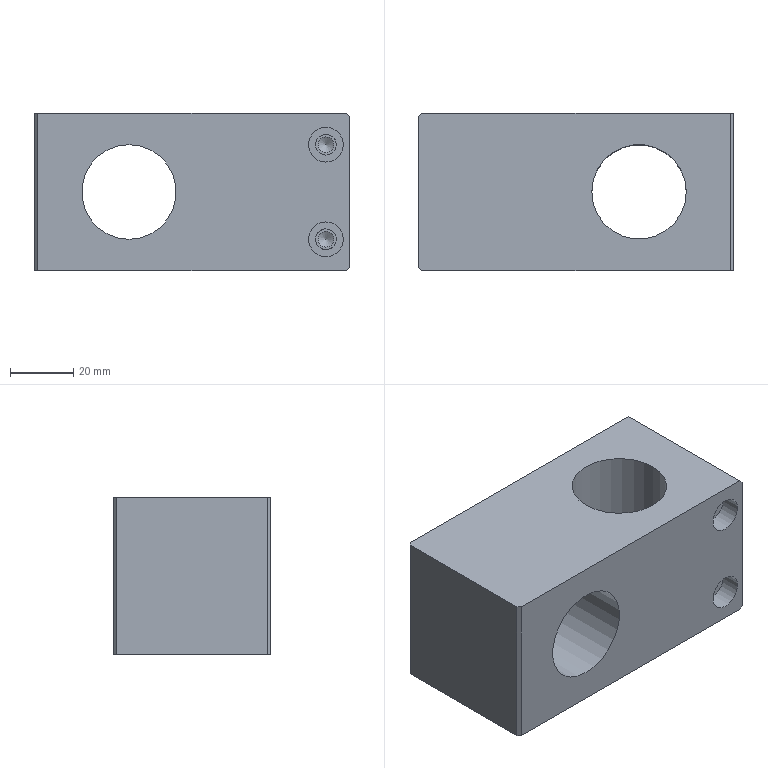Part | NX | 1 solid | 36 faces | box 100 x 50 x 50 mm | volume 172813 mm3 | plane 18 | cylinder 14 | cone 4 | commonest cylinder face diameters 5 x4 6.6 x4 11 x4 30 x2
STEP:
#1=CARTESIAN_POINT('',(42.5,1.5,7.5));
#2=VERTEX_POINT('',#1);
#3=CARTESIAN_POINT('',(42.5,1.5,10.));
#4=DIRECTION('',(0.,-1.,0.));
#5=DIRECTION('',(0.,0.,-1.));
#6=AXIS2_PLACEMENT_3D('',#3,#4,#5);
#7=CIRCLE('',#6,2.5);
#8=EDGE_CURVE('',#2,#2,#7,.T.);
#9=ORIENTED_EDGE('',*,*,#8,.F.);
#10=EDGE_LOOP('',(#9));
#11=FACE_BOUND('',#10,.T.);
#12=CARTESIAN_POINT('',(39.2,1.5,10.));
#13=VERTEX_POINT('',#12);
#14=CARTESIAN_POINT('',(42.5,1.5,10.));
#15=DIRECTION('',(0.,1.,0.));
#16=DIRECTION('',(-1.,0.,0.));
#17=AXIS2_PLACEMENT_3D('',#14,#15,#16);
#18=CIRCLE('',#17,3.3);
#19=EDGE_CURVE('',#13,#13,#18,.T.);
#20=ORIENTED_EDGE('',*,*,#19,.F.);
#21=EDGE_LOOP('',(#20));
#22=FACE_BOUND('',#21,.T.);
#23=CARTESIAN_POINT('',(0.,1.5,50.));
#24=DIRECTION('',(0.,1.,0.));
#25=DIRECTION('',(-1.,0.,0.));
#26=AXIS2_PLACEMENT_3D('',#23,#24,#25);
#27=PLANE('',#26);
#28=ADVANCED_FACE('',(#11,#22),#27,.F.);
#29=CARTESIAN_POINT('',(42.5,1.5,37.5));
#30=VERTEX_POINT('',#29);
#31=CARTESIAN_POINT('',(42.5,1.5,40.));
#32=DIRECTION('',(0.,-1.,0.));
#33=DIRECTION('',(0.,0.,-1.));
#34=AXIS2_PLACEMENT_3D('',#31,#32,#33);
#35=CIRCLE('',#34,2.5);
#36=EDGE_CURVE('',#30,#30,#35,.T.);
#37=ORIENTED_EDGE('',*,*,#36,.F.);
#38=EDGE_LOOP('',(#37));
#39=FACE_BOUND('',#38,.T.);
#40=CARTESIAN_POINT('',(39.2,1.5,40.));
#41=VERTEX_POINT('',#40);
#42=CARTESIAN_POINT('',(42.5,1.5,40.));
#43=DIRECTION('',(0.,1.,0.));
#44=DIRECTION('',(-1.,0.,0.));
#45=AXIS2_PLACEMENT_3D('',#42,#43,#44);
#46=CIRCLE('',#45,3.3);
#47=EDGE_CURVE('',#41,#41,#46,.T.);
#48=ORIENTED_EDGE('',*,*,#47,.F.);
#49=EDGE_LOOP('',(#48));
#50=FACE_BOUND('',#49,.T.);
#51=CARTESIAN_POINT('',(0.,1.5,50.));
#52=DIRECTION('',(0.,1.,0.));
#53=DIRECTION('',(-1.,0.,0.));
#54=AXIS2_PLACEMENT_3D('',#51,#52,#53);
#55=PLANE('',#54);
#56=ADVANCED_FACE('',(#39,#50),#55,.F.);
#57=CARTESIAN_POINT('',(-45.,15.,26.5));
#58=VERTEX_POINT('',#57);
#59=CARTESIAN_POINT('',(-42.5,15.,26.5));
#60=DIRECTION('',(0.,0.,-1.));
#61=DIRECTION('',(-1.,0.,0.));
#62=AXIS2_PLACEMENT_3D('',#59,#60,#61);
#63=CIRCLE('',#62,2.5);
#64=EDGE_CURVE('',#58,#58,#63,.T.);
#65=ORIENTED_EDGE('',*,*,#64,.F.);
#66=EDGE_LOOP('',(#65));
#67=FACE_BOUND('',#66,.T.);
#68=CARTESIAN_POINT('',(-39.2,15.,26.5));
#69=VERTEX_POINT('',#68);
#70=CARTESIAN_POINT('',(-42.5,15.,26.5));
#71=DIRECTION('',(0.,0.,1.));
#72=DIRECTION('',(1.,0.,0.));
#73=AXIS2_PLACEMENT_3D('',#70,#71,#72);
#74=CIRCLE('',#73,3.3);
#75=EDGE_CURVE('',#69,#69,#74,.F.);
#76=ORIENTED_EDGE('',*,*,#75,.T.);
#77=EDGE_LOOP('',(#76));
#78=FACE_BOUND('',#77,.T.);
#79=CARTESIAN_POINT('',(-50.,25.,26.5));
#80=DIRECTION('',(0.,0.,1.));
#81=DIRECTION('',(1.,0.,0.));
#82=AXIS2_PLACEMENT_3D('',#79,#80,#81);
#83=PLANE('',#82);
#84=ADVANCED_FACE('',(#67,#78),#83,.F.);
#85=CARTESIAN_POINT('',(-45.,-15.,26.5));
#86=VERTEX_POINT('',#85);
#87=CARTESIAN_POINT('',(-42.5,-15.,26.5));
#88=DIRECTION('',(0.,0.,-1.));
#89=DIRECTION('',(-1.,0.,0.));
#90=AXIS2_PLACEMENT_3D('',#87,#88,#89);
#91=CIRCLE('',#90,2.5);
#92=EDGE_CURVE('',#86,#86,#91,.T.);
#93=ORIENTED_EDGE('',*,*,#92,.F.);
#94=EDGE_LOOP('',(#93));
#95=FACE_BOUND('',#94,.T.);
#96=CARTESIAN_POINT('',(-39.2,-15.,26.5));
#97=VERTEX_POINT('',#96);
#98=CARTESIAN_POINT('',(-42.5,-15.,26.5));
#99=DIRECTION('',(0.,0.,1.));
#100=DIRECTION('',(1.,0.,0.));
#101=AXIS2_PLACEMENT_3D('',#98,#99,#100);
#102=CIRCLE('',#101,3.3);
#103=EDGE_CURVE('',#97,#97,#102,.F.);
#104=ORIENTED_EDGE('',*,*,#103,.T.);
#105=EDGE_LOOP('',(#104));
#106=FACE_BOUND('',#105,.T.);
#107=CARTESIAN_POINT('',(-50.,25.,26.5));
#108=DIRECTION('',(0.,0.,1.));
#109=DIRECTION('',(1.,0.,0.));
#110=AXIS2_PLACEMENT_3D('',#107,#108,#109);
#111=PLANE('',#110);
#112=ADVANCED_FACE('',(#95,#106),#111,.F.);
#113=CARTESIAN_POINT('',(-50.,24.,0.));
#114=VERTEX_POINT('',#113);
#115=CARTESIAN_POINT('',(-49.,25.,0.));
#116=VERTEX_POINT('',#115);
#117=CARTESIAN_POINT('',(-37.,37.,0.));
#118=DIRECTION('',(0.7071,0.7071,0.));
#119=VECTOR('',#118,1000.);
#120=LINE('',#117,#119);
#121=EDGE_CURVE('',#114,#116,#120,.T.);
#122=ORIENTED_EDGE('',*,*,#121,.F.);
#123=CARTESIAN_POINT('',(-50.,24.,50.));
#124=VERTEX_POINT('',#123);
#125=CARTESIAN_POINT('',(-50.,24.,50.));
#126=DIRECTION('',(0.,0.,-1.));
#127=VECTOR('',#126,1000.);
#128=LINE('',#125,#127);
#129=EDGE_CURVE('',#124,#114,#128,.T.);
#130=ORIENTED_EDGE('',*,*,#129,.F.);
#131=CARTESIAN_POINT('',(-49.,25.,50.));
#132=VERTEX_POINT('',#131);
#133=CARTESIAN_POINT('',(-50.,24.,50.));
#134=DIRECTION('',(-0.7071,-0.7071,0.));
#135=VECTOR('',#134,1000.);
#136=LINE('',#133,#135);
#137=EDGE_CURVE('',#132,#124,#136,.T.);
#138=ORIENTED_EDGE('',*,*,#137,.F.);
#139=CARTESIAN_POINT('',(-49.,25.,50.));
#140=DIRECTION('',(0.,0.,1.));
#141=VECTOR('',#140,1000.);
#142=LINE('',#139,#141);
#143=EDGE_CURVE('',#116,#132,#142,.T.);
#144=ORIENTED_EDGE('',*,*,#143,.F.);
#145=EDGE_LOOP('',(#122,#130,#138,#144));
#146=FACE_BOUND('',#145,.T.);
#147=CARTESIAN_POINT('',(-50.,24.,50.));
#148=DIRECTION('',(0.7071,-0.7071,0.));
#149=DIRECTION('',(0.,0.,-1.));
#150=AXIS2_PLACEMENT_3D('',#147,#148,#149);
#151=PLANE('',#150);
#152=ADVANCED_FACE('',(#146),#151,.F.);
#153=CARTESIAN_POINT('',(-49.,-25.,0.));
#154=VERTEX_POINT('',#153);
#155=CARTESIAN_POINT('',(-50.,-24.,0.));
#156=VERTEX_POINT('',#155);
#157=CARTESIAN_POINT('',(-37.,-37.,0.));
#158=DIRECTION('',(-0.7071,0.7071,0.));
#159=VECTOR('',#158,1000.);
#160=LINE('',#157,#159);
#161=EDGE_CURVE('',#154,#156,#160,.T.);
#162=ORIENTED_EDGE('',*,*,#161,.F.);
#163=CARTESIAN_POINT('',(-49.,-25.,50.));
#164=VERTEX_POINT('',#163);
#165=CARTESIAN_POINT('',(-49.,-25.,50.));
#166=DIRECTION('',(0.,0.,-1.));
#167=VECTOR('',#166,1000.);
#168=LINE('',#165,#167);
#169=EDGE_CURVE('',#164,#154,#168,.T.);
#170=ORIENTED_EDGE('',*,*,#169,.F.);
#171=CARTESIAN_POINT('',(-50.,-24.,50.));
#172=VERTEX_POINT('',#171);
#173=CARTESIAN_POINT('',(-49.,-25.,50.));
#174=DIRECTION('',(0.7071,-0.7071,0.));
#175=VECTOR('',#174,1000.);
#176=LINE('',#173,#175);
#177=EDGE_CURVE('',#172,#164,#176,.T.);
#178=ORIENTED_EDGE('',*,*,#177,.F.);
#179=CARTESIAN_POINT('',(-50.,-24.,50.));
#180=DIRECTION('',(0.,0.,1.));
#181=VECTOR('',#180,1000.);
#182=LINE('',#179,#181);
#183=EDGE_CURVE('',#156,#172,#182,.T.);
#184=ORIENTED_EDGE('',*,*,#183,.F.);
#185=EDGE_LOOP('',(#162,#170,#178,#184));
#186=FACE_BOUND('',#185,.T.);
#187=CARTESIAN_POINT('',(-49.,-25.,50.));
#188=DIRECTION('',(0.7071,0.7071,0.));
#189=DIRECTION('',(0.,0.,-1.));
#190=AXIS2_PLACEMENT_3D('',#187,#188,#189);
#191=PLANE('',#190);
#192=ADVANCED_FACE('',(#186),#191,.F.);
#193=CARTESIAN_POINT('',(49.,-25.,50.));
#194=VERTEX_POINT('',#193);
#195=CARTESIAN_POINT('',(49.,25.,50.));
#196=VERTEX_POINT('',#195);
#197=CARTESIAN_POINT('',(49.,0.,50.));
#198=DIRECTION('',(0.,1.,0.));
#199=VECTOR('',#198,1000.);
#200=LINE('',#197,#199);
#201=EDGE_CURVE('',#194,#196,#200,.T.);
#202=ORIENTED_EDGE('',*,*,#201,.F.);
#203=CARTESIAN_POINT('',(50.,-25.,49.));
#204=VERTEX_POINT('',#203);
#205=CARTESIAN_POINT('',(49.,-25.,50.));
#206=DIRECTION('',(-0.7071,0.,0.7071));
#207=VECTOR('',#206,1000.);
#208=LINE('',#205,#207);
#209=EDGE_CURVE('',#204,#194,#208,.T.);
#210=ORIENTED_EDGE('',*,*,#209,.F.);
#211=CARTESIAN_POINT('',(50.,25.,49.));
#212=VERTEX_POINT('',#211);
#213=CARTESIAN_POINT('',(50.,-25.,49.));
#214=DIRECTION('',(0.,-1.,0.));
#215=VECTOR('',#214,1000.);
#216=LINE('',#213,#215);
#217=EDGE_CURVE('',#212,#204,#216,.T.);
#218=ORIENTED_EDGE('',*,*,#217,.F.);
#219=CARTESIAN_POINT('',(49.,25.,50.));
#220=DIRECTION('',(0.7071,0.,-0.7071));
#221=VECTOR('',#220,1000.);
#222=LINE('',#219,#221);
#223=EDGE_CURVE('',#196,#212,#222,.T.);
#224=ORIENTED_EDGE('',*,*,#223,.F.);
#225=EDGE_LOOP('',(#202,#210,#218,#224));
#226=FACE_BOUND('',#225,.T.);
#227=CARTESIAN_POINT('',(49.,0.,50.));
#228=DIRECTION('',(-0.7071,0.,-0.7071));
#229=DIRECTION('',(0.,1.,0.));
#230=AXIS2_PLACEMENT_3D('',#227,#228,#229);
#231=PLANE('',#230);
#232=ADVANCED_FACE('',(#226),#231,.F.);
#233=CARTESIAN_POINT('',(49.,-25.,0.));
#234=VERTEX_POINT('',#233);
#235=CARTESIAN_POINT('',(50.,-25.,1.));
#236=VERTEX_POINT('',#235);
#237=CARTESIAN_POINT('',(50.,-25.,1.));
#238=DIRECTION('',(0.7071,0.,0.7071));
#239=VECTOR('',#238,1000.);
#240=LINE('',#237,#239);
#241=EDGE_CURVE('',#234,#236,#240,.T.);
#242=ORIENTED_EDGE('',*,*,#241,.F.);
#243=CARTESIAN_POINT('',(49.,25.,0.));
#244=VERTEX_POINT('',#243);
#245=CARTESIAN_POINT('',(49.,-25.,0.));
#246=DIRECTION('',(0.,-1.,0.));
#247=VECTOR('',#246,1000.);
#248=LINE('',#245,#247);
#249=EDGE_CURVE('',#244,#234,#248,.T.);
#250=ORIENTED_EDGE('',*,*,#249,.F.);
#251=CARTESIAN_POINT('',(50.,25.,1.));
#252=VERTEX_POINT('',#251);
#253=CARTESIAN_POINT('',(50.,25.,1.));
#254=DIRECTION('',(-0.7071,0.,-0.7071));
#255=VECTOR('',#254,1000.);
#256=LINE('',#253,#255);
#257=EDGE_CURVE('',#252,#244,#256,.T.);
#258=ORIENTED_EDGE('',*,*,#257,.F.);
#259=CARTESIAN_POINT('',(50.,-1.5,1.));
#260=DIRECTION('',(0.,1.,0.));
#261=VECTOR('',#260,1000.);
#262=LINE('',#259,#261);
#263=EDGE_CURVE('',#236,#252,#262,.T.);
#264=ORIENTED_EDGE('',*,*,#263,.F.);
#265=EDGE_LOOP('',(#242,#250,#258,#264));
#266=FACE_BOUND('',#265,.T.);
#267=CARTESIAN_POINT('',(50.,-25.,1.));
#268=DIRECTION('',(0.7071,0.,-0.7071));
#269=DIRECTION('',(0.,-1.,0.));
#270=AXIS2_PLACEMENT_3D('',#267,#268,#269);
#271=PLANE('',#270);
#272=ADVANCED_FACE('',(#266),#271,.T.);
#273=CARTESIAN_POINT('',(-48.,15.,6.4));
#274=VERTEX_POINT('',#273);
#275=CARTESIAN_POINT('',(-42.5,15.,6.4));
#276=DIRECTION('',(0.,0.,-1.));
#277=DIRECTION('',(-1.,0.,0.));
#278=AXIS2_PLACEMENT_3D('',#275,#276,#277);
#279=CIRCLE('',#278,5.5);
#280=EDGE_CURVE('',#274,#274,#279,.T.);
#281=ORIENTED_EDGE('',*,*,#280,.T.);
#282=EDGE_LOOP('',(#281));
#283=FACE_BOUND('',#282,.T.);
#284=CARTESIAN_POINT('',(-45.8,15.,6.4));
#285=VERTEX_POINT('',#284);
#286=CARTESIAN_POINT('',(-42.5,15.,6.4));
#287=DIRECTION('',(0.,0.,-1.));
#288=DIRECTION('',(-1.,0.,0.));
#289=AXIS2_PLACEMENT_3D('',#286,#287,#288);
#290=CIRCLE('',#289,3.3);
#291=EDGE_CURVE('',#285,#285,#290,.T.);
#292=ORIENTED_EDGE('',*,*,#291,.F.);
#293=EDGE_LOOP('',(#292));
#294=FACE_BOUND('',#293,.T.);
#295=CARTESIAN_POINT('',(-39.2,15.,6.4));
#296=DIRECTION('',(0.,0.,1.));
#297=DIRECTION('',(1.,0.,0.));
#298=AXIS2_PLACEMENT_3D('',#295,#296,#297);
#299=PLANE('',#298);
#300=ADVANCED_FACE('',(#283,#294),#299,.F.);
#301=CARTESIAN_POINT('',(-37.,-15.,6.4));
#302=VERTEX_POINT('',#301);
#303=CARTESIAN_POINT('',(-42.5,-15.,6.4));
#304=DIRECTION('',(0.,0.,-1.));
#305=DIRECTION('',(1.,0.,0.));
#306=AXIS2_PLACEMENT_3D('',#303,#304,#305);
#307=CIRCLE('',#306,5.5);
#308=EDGE_CURVE('',#302,#302,#307,.T.);
#309=ORIENTED_EDGE('',*,*,#308,.T.);
#310=EDGE_LOOP('',(#309));
#311=FACE_BOUND('',#310,.T.);
#312=CARTESIAN_POINT('',(-39.2,-15.,6.4));
#313=VERTEX_POINT('',#312);
#314=CARTESIAN_POINT('',(-42.5,-15.,6.4));
#315=DIRECTION('',(0.,0.,-1.));
#316=DIRECTION('',(1.,0.,0.));
#317=AXIS2_PLACEMENT_3D('',#314,#315,#316);
#318=CIRCLE('',#317,3.3);
#319=EDGE_CURVE('',#313,#313,#318,.T.);
#320=ORIENTED_EDGE('',*,*,#319,.F.);
#321=EDGE_LOOP('',(#320));
#322=FACE_BOUND('',#321,.T.);
#323=CARTESIAN_POINT('',(-39.2,15.,6.4));
#324=DIRECTION('',(0.,0.,1.));
#325=DIRECTION('',(1.,0.,0.));
#326=AXIS2_PLACEMENT_3D('',#323,#324,#325);
#327=PLANE('',#326);
#328=ADVANCED_FACE('',(#311,#322),#327,.F.);
#329=CARTESIAN_POINT('',(42.5,-18.6,34.5));
#330=VERTEX_POINT('',#329);
#331=CARTESIAN_POINT('',(42.5,-18.6,40.));
#332=DIRECTION('',(0.,-1.,0.));
#333=DIRECTION('',(0.,0.,-1.));
#334=AXIS2_PLACEMENT_3D('',#331,#332,#333);
#335=CIRCLE('',#334,5.5);
#336=EDGE_CURVE('',#330,#330,#335,.T.);
#337=ORIENTED_EDGE('',*,*,#336,.T.);
#338=EDGE_LOOP('',(#337));
#339=FACE_BOUND('',#338,.T.);
#340=CARTESIAN_POINT('',(42.5,-18.6,36.7));
#341=VERTEX_POINT('',#340);
#342=CARTESIAN_POINT('',(42.5,-18.6,40.));
#343=DIRECTION('',(0.,-1.,0.));
#344=DIRECTION('',(0.,0.,-1.));
#345=AXIS2_PLACEMENT_3D('',#342,#343,#344);
#346=CIRCLE('',#345,3.3);
#347=EDGE_CURVE('',#341,#341,#346,.T.);
#348=ORIENTED_EDGE('',*,*,#347,.F.);
#349=EDGE_LOOP('',(#348));
#350=FACE_BOUND('',#349,.T.);
#351=CARTESIAN_POINT('',(45.8,-18.6,40.));
#352=DIRECTION('',(0.,1.,0.));
#353=DIRECTION('',(0.,0.,1.));
#354=AXIS2_PLACEMENT_3D('',#351,#352,#353);
#355=PLANE('',#354);
#356=ADVANCED_FACE('',(#339,#350),#355,.F.);
#357=CARTESIAN_POINT('',(42.5,-18.6,15.5));
#358=VERTEX_POINT('',#357);
#359=CARTESIAN_POINT('',(42.5,-18.6,10.));
#360=DIRECTION('',(0.,-1.,0.));
#361=DIRECTION('',(0.,0.,1.));
#362=AXIS2_PLACEMENT_3D('',#359,#360,#361);
#363=CIRCLE('',#362,5.5);
#364=EDGE_CURVE('',#358,#358,#363,.T.);
#365=ORIENTED_EDGE('',*,*,#364,.T.);
#366=EDGE_LOOP('',(#365));
#367=FACE_BOUND('',#366,.T.);
#368=CARTESIAN_POINT('',(42.5,-18.6,13.3));
#369=VERTEX_POINT('',#368);
#370=CARTESIAN_POINT('',(42.5,-18.6,10.));
#371=DIRECTION('',(0.,-1.,0.));
#372=DIRECTION('',(0.,0.,1.));
#373=AXIS2_PLACEMENT_3D('',#370,#371,#372);
#374=CIRCLE('',#373,3.3);
#375=EDGE_CURVE('',#369,#369,#374,.T.);
#376=ORIENTED_EDGE('',*,*,#375,.F.);
#377=EDGE_LOOP('',(#376));
#378=FACE_BOUND('',#377,.T.);
#379=CARTESIAN_POINT('',(45.8,-18.6,40.));
#380=DIRECTION('',(0.,1.,0.));
#381=DIRECTION('',(0.,0.,1.));
#382=AXIS2_PLACEMENT_3D('',#379,#380,#381);
#383=PLANE('',#382);
#384=ADVANCED_FACE('',(#367,#378),#383,.F.);
#385=CARTESIAN_POINT('',(-50.,25.,0.));
#386=DIRECTION('',(-1.,0.,0.));
#387=VECTOR('',#386,1000.);
#388=LINE('',#385,#387);
#389=EDGE_CURVE('',#244,#116,#388,.T.);
#390=ORIENTED_EDGE('',*,*,#389,.F.);
#391=ORIENTED_EDGE('',*,*,#249,.T.);
#392=CARTESIAN_POINT('',(-50.,-25.,0.));
#393=DIRECTION('',(1.,0.,0.));
#394=VECTOR('',#393,1000.);
#395=LINE('',#392,#394);
#396=EDGE_CURVE('',#154,#234,#395,.T.);
#397=ORIENTED_EDGE('',*,*,#396,.F.);
#398=ORIENTED_EDGE('',*,*,#161,.T.);
#399=CARTESIAN_POINT('',(-50.,-25.,0.));
#400=DIRECTION('',(0.,-1.,0.));
#401=VECTOR('',#400,1000.);
#402=LINE('',#399,#401);
#403=EDGE_CURVE('',#114,#156,#402,.T.);
#404=ORIENTED_EDGE('',*,*,#403,.F.);
#405=ORIENTED_EDGE('',*,*,#121,.T.);
#406=EDGE_LOOP('',(#390,#391,#397,#398,#404,#405));
#407=FACE_BOUND('',#406,.T.);
#408=CARTESIAN_POINT('',(35.,0.,0.));
#409=VERTEX_POINT('',#408);
#410=CARTESIAN_POINT('',(20.,0.,0.));
#411=DIRECTION('',(0.,0.,1.));
#412=DIRECTION('',(1.,0.,0.));
#413=AXIS2_PLACEMENT_3D('',#410,#411,#412);
#414=CIRCLE('',#413,15.);
#415=EDGE_CURVE('',#409,#409,#414,.T.);
#416=ORIENTED_EDGE('',*,*,#415,.T.);
#417=EDGE_LOOP('',(#416));
#418=FACE_BOUND('',#417,.T.);
#419=CARTESIAN_POINT('',(-48.,-15.,0.));
#420=VERTEX_POINT('',#419);
#421=CARTESIAN_POINT('',(-42.5,-15.,0.));
#422=DIRECTION('',(0.,0.,-1.));
#423=DIRECTION('',(-1.,0.,0.));
#424=AXIS2_PLACEMENT_3D('',#421,#422,#423);
#425=CIRCLE('',#424,5.5);
#426=EDGE_CURVE('',#420,#420,#425,.T.);
#427=ORIENTED_EDGE('',*,*,#426,.F.);
#428=EDGE_LOOP('',(#427));
#429=FACE_BOUND('',#428,.T.);
#430=CARTESIAN_POINT('',(-48.,15.,0.));
#431=VERTEX_POINT('',#430);
#432=CARTESIAN_POINT('',(-42.5,15.,0.));
#433=DIRECTION('',(0.,0.,-1.));
#434=DIRECTION('',(-1.,0.,0.));
#435=AXIS2_PLACEMENT_3D('',#432,#433,#434);
#436=CIRCLE('',#435,5.5);
#437=EDGE_CURVE('',#431,#431,#436,.T.);
#438=ORIENTED_EDGE('',*,*,#437,.F.);
#439=EDGE_LOOP('',(#438));
#440=FACE_BOUND('',#439,.T.);
#441=CARTESIAN_POINT('',(0.,0.,0.));
#442=DIRECTION('',(0.,0.,-1.));
#443=DIRECTION('',(-1.,0.,0.));
#444=AXIS2_PLACEMENT_3D('',#441,#442,#443);
#445=PLANE('',#444);
#446=ADVANCED_FACE('',(#407,#418,#429,#440),#445,.T.);
#447=CARTESIAN_POINT('',(-50.,-25.,50.));
#448=DIRECTION('',(1.,0.,0.));
#449=VECTOR('',#448,1000.);
#450=LINE('',#447,#449);
#451=EDGE_CURVE('',#164,#194,#450,.T.);
#452=ORIENTED_EDGE('',*,*,#451,.T.);
#453=ORIENTED_EDGE('',*,*,#201,.T.);
#454=CARTESIAN_POINT('',(-50.,25.,50.));
#455=DIRECTION('',(-1.,0.,0.));
#456=VECTOR('',#455,1000.);
#457=LINE('',#454,#456);
#458=EDGE_CURVE('',#196,#132,#457,.T.);
#459=ORIENTED_EDGE('',*,*,#458,.T.);
#460=ORIENTED_EDGE('',*,*,#137,.T.);
#461=CARTESIAN_POINT('',(-50.,-25.,50.));
#462=DIRECTION('',(0.,-1.,0.));
#463=VECTOR('',#462,1000.);
#464=LINE('',#461,#463);
#465=EDGE_CURVE('',#124,#172,#464,.T.);
#466=ORIENTED_EDGE('',*,*,#465,.T.);
#467=ORIENTED_EDGE('',*,*,#177,.T.);
#468=EDGE_LOOP('',(#452,#453,#459,#460,#466,#467));
#469=FACE_BOUND('',#468,.T.);
#470=CARTESIAN_POINT('',(35.,0.,50.));
#471=VERTEX_POINT('',#470);
#472=CARTESIAN_POINT('',(20.,0.,50.));
#473=DIRECTION('',(0.,0.,1.));
#474=DIRECTION('',(1.,0.,0.));
#475=AXIS2_PLACEMENT_3D('',#472,#473,#474);
#476=CIRCLE('',#475,15.);
#477=EDGE_CURVE('',#471,#471,#476,.T.);
#478=ORIENTED_EDGE('',*,*,#477,.F.);
#479=EDGE_LOOP('',(#478));
#480=FACE_BOUND('',#479,.T.);
#481=CARTESIAN_POINT('',(0.,0.,50.));
#482=DIRECTION('',(0.,0.,-1.));
#483=DIRECTION('',(-1.,0.,0.));
#484=AXIS2_PLACEMENT_3D('',#481,#482,#483);
#485=PLANE('',#484);
#486=ADVANCED_FACE('',(#469,#480),#485,.F.);
#487=CARTESIAN_POINT('',(-20.,-25.,40.));
#488=VERTEX_POINT('',#487);
#489=CARTESIAN_POINT('',(-20.,-25.,25.));
#490=DIRECTION('',(0.,1.,0.));
#491=DIRECTION('',(0.,0.,1.));
#492=AXIS2_PLACEMENT_3D('',#489,#490,#491);
#493=CIRCLE('',#492,15.);
#494=EDGE_CURVE('',#488,#488,#493,.T.);
#495=ORIENTED_EDGE('',*,*,#494,.T.);
#496=EDGE_LOOP('',(#495));
#497=FACE_BOUND('',#496,.T.);
#498=ORIENTED_EDGE('',*,*,#396,.T.);
#499=ORIENTED_EDGE('',*,*,#241,.T.);
#500=CARTESIAN_POINT('',(50.,-25.,50.));
#501=DIRECTION('',(0.,0.,-1.));
#502=VECTOR('',#501,1000.);
#503=LINE('',#500,#502);
#504=EDGE_CURVE('',#204,#236,#503,.T.);
#505=ORIENTED_EDGE('',*,*,#504,.F.);
#506=ORIENTED_EDGE('',*,*,#209,.T.);
#507=ORIENTED_EDGE('',*,*,#451,.F.);
#508=ORIENTED_EDGE('',*,*,#169,.T.);
#509=EDGE_LOOP('',(#498,#499,#505,#506,#507,#508));
#510=FACE_BOUND('',#509,.T.);
#511=CARTESIAN_POINT('',(42.5,-25.,4.5));
#512=VERTEX_POINT('',#511);
#513=CARTESIAN_POINT('',(42.5,-25.,10.));
#514=DIRECTION('',(0.,-1.,0.));
#515=DIRECTION('',(0.,0.,-1.));
#516=AXIS2_PLACEMENT_3D('',#513,#514,#515);
#517=CIRCLE('',#516,5.5);
#518=EDGE_CURVE('',#512,#512,#517,.T.);
#519=ORIENTED_EDGE('',*,*,#518,.F.);
#520=EDGE_LOOP('',(#519));
#521=FACE_BOUND('',#520,.T.);
#522=CARTESIAN_POINT('',(42.5,-25.,34.5));
#523=VERTEX_POINT('',#522);
#524=CARTESIAN_POINT('',(42.5,-25.,40.));
#525=DIRECTION('',(0.,-1.,0.));
#526=DIRECTION('',(0.,0.,-1.));
#527=AXIS2_PLACEMENT_3D('',#524,#525,#526);
#528=CIRCLE('',#527,5.5);
#529=EDGE_CURVE('',#523,#523,#528,.T.);
#530=ORIENTED_EDGE('',*,*,#529,.F.);
#531=EDGE_LOOP('',(#530));
#532=FACE_BOUND('',#531,.T.);
#533=CARTESIAN_POINT('',(-50.,-25.,50.));
#534=DIRECTION('',(0.,1.,0.));
#535=DIRECTION('',(0.,0.,1.));
#536=AXIS2_PLACEMENT_3D('',#533,#534,#535);
#537=PLANE('',#536);
#538=ADVANCED_FACE('',(#497,#510,#521,#532),#537,.F.);
#539=CARTESIAN_POINT('',(-20.,25.,40.));
#540=VERTEX_POINT('',#539);
#541=CARTESIAN_POINT('',(-20.,25.,25.));
#542=DIRECTION('',(0.,1.,0.));
#543=DIRECTION('',(0.,0.,1.));
#544=AXIS2_PLACEMENT_3D('',#541,#542,#543);
#545=CIRCLE('',#544,15.);
#546=EDGE_CURVE('',#540,#540,#545,.T.);
#547=ORIENTED_EDGE('',*,*,#546,.F.);
#548=EDGE_LOOP('',(#547));
#549=FACE_BOUND('',#548,.T.);
#550=CARTESIAN_POINT('',(50.,25.,50.));
#551=DIRECTION('',(0.,0.,-1.));
#552=VECTOR('',#551,1000.);
#553=LINE('',#550,#552);
#554=EDGE_CURVE('',#212,#252,#553,.T.);
#555=ORIENTED_EDGE('',*,*,#554,.T.);
#556=ORIENTED_EDGE('',*,*,#257,.T.);
#557=ORIENTED_EDGE('',*,*,#389,.T.);
#558=ORIENTED_EDGE('',*,*,#143,.T.);
#559=ORIENTED_EDGE('',*,*,#458,.F.);
#560=ORIENTED_EDGE('',*,*,#223,.T.);
#561=EDGE_LOOP('',(#555,#556,#557,#558,#559,#560));
#562=FACE_BOUND('',#561,.T.);
#563=CARTESIAN_POINT('',(-50.,25.,50.));
#564=DIRECTION('',(0.,-1.,0.));
#565=DIRECTION('',(0.,0.,-1.));
#566=AXIS2_PLACEMENT_3D('',#563,#564,#565);
#567=PLANE('',#566);
#568=ADVANCED_FACE('',(#549,#562),#567,.F.);
#569=ORIENTED_EDGE('',*,*,#465,.F.);
#570=ORIENTED_EDGE('',*,*,#129,.T.);
#571=ORIENTED_EDGE('',*,*,#403,.T.);
#572=ORIENTED_EDGE('',*,*,#183,.T.);
#573=EDGE_LOOP('',(#569,#570,#571,#572));
#574=FACE_BOUND('',#573,.T.);
#575=CARTESIAN_POINT('',(-50.,-25.,50.));
#576=DIRECTION('',(1.,0.,0.));
#577=DIRECTION('',(0.,0.,-1.));
#578=AXIS2_PLACEMENT_3D('',#575,#576,#577);
#579=PLANE('',#578);
#580=ADVANCED_FACE('',(#574),#579,.F.);
#581=ORIENTED_EDGE('',*,*,#415,.F.);
#582=EDGE_LOOP('',(#581));
#583=FACE_BOUND('',#582,.T.);
#584=ORIENTED_EDGE('',*,*,#477,.T.);
#585=EDGE_LOOP('',(#584));
#586=FACE_BOUND('',#585,.T.);
#587=CARTESIAN_POINT('',(20.,0.,0.));
#588=DIRECTION('',(0.,0.,1.));
#589=DIRECTION('',(1.,0.,0.));
#590=AXIS2_PLACEMENT_3D('',#587,#588,#589);
#591=CYLINDRICAL_SURFACE('',#590,15.);
#592=ADVANCED_FACE('',(#583,#586),#591,.F.);
#593=ORIENTED_EDGE('',*,*,#504,.T.);
#594=ORIENTED_EDGE('',*,*,#263,.T.);
#595=ORIENTED_EDGE('',*,*,#554,.F.);
#596=ORIENTED_EDGE('',*,*,#217,.T.);
#597=EDGE_LOOP('',(#593,#594,#595,#596));
#598=FACE_BOUND('',#597,.T.);
#599=CARTESIAN_POINT('',(50.,-25.,50.));
#600=DIRECTION('',(-1.,0.,0.));
#601=DIRECTION('',(0.,0.,1.));
#602=AXIS2_PLACEMENT_3D('',#599,#600,#601);
#603=PLANE('',#602);
#604=ADVANCED_FACE('',(#598),#603,.F.);
#605=ORIENTED_EDGE('',*,*,#546,.T.);
#606=EDGE_LOOP('',(#605));
#607=FACE_BOUND('',#606,.T.);
#608=ORIENTED_EDGE('',*,*,#494,.F.);
#609=EDGE_LOOP('',(#608));
#610=FACE_BOUND('',#609,.T.);
#611=CARTESIAN_POINT('',(-20.,-25.,25.));
#612=DIRECTION('',(0.,1.,0.));
#613=DIRECTION('',(0.,0.,1.));
#614=AXIS2_PLACEMENT_3D('',#611,#612,#613);
#615=CYLINDRICAL_SURFACE('',#614,15.);
#616=ADVANCED_FACE('',(#607,#610),#615,.F.);
#617=ORIENTED_EDGE('',*,*,#375,.T.);
#618=EDGE_LOOP('',(#617));
#619=FACE_BOUND('',#618,.T.);
#620=ORIENTED_EDGE('',*,*,#19,.T.);
#621=EDGE_LOOP('',(#620));
#622=FACE_BOUND('',#621,.T.);
#623=CARTESIAN_POINT('',(42.5,-25.,10.));
#624=DIRECTION('',(0.,-1.,0.));
#625=DIRECTION('',(0.,0.,-1.));
#626=AXIS2_PLACEMENT_3D('',#623,#624,#625);
#627=CYLINDRICAL_SURFACE('',#626,3.3);
#628=ADVANCED_FACE('',(#619,#622),#627,.F.);
#629=ORIENTED_EDGE('',*,*,#518,.T.);
#630=EDGE_LOOP('',(#629));
#631=FACE_BOUND('',#630,.T.);
#632=ORIENTED_EDGE('',*,*,#364,.F.);
#633=EDGE_LOOP('',(#632));
#634=FACE_BOUND('',#633,.T.);
#635=CARTESIAN_POINT('',(42.5,-25.,10.));
#636=DIRECTION('',(0.,-1.,0.));
#637=DIRECTION('',(0.,0.,-1.));
#638=AXIS2_PLACEMENT_3D('',#635,#636,#637);
#639=CYLINDRICAL_SURFACE('',#638,5.5);
#640=ADVANCED_FACE('',(#631,#634),#639,.F.);
#641=ORIENTED_EDGE('',*,*,#347,.T.);
#642=EDGE_LOOP('',(#641));
#643=FACE_BOUND('',#642,.T.);
#644=ORIENTED_EDGE('',*,*,#47,.T.);
#645=EDGE_LOOP('',(#644));
#646=FACE_BOUND('',#645,.T.);
#647=CARTESIAN_POINT('',(42.5,-25.,40.));
#648=DIRECTION('',(0.,-1.,0.));
#649=DIRECTION('',(0.,0.,-1.));
#650=AXIS2_PLACEMENT_3D('',#647,#648,#649);
#651=CYLINDRICAL_SURFACE('',#650,3.3);
#652=ADVANCED_FACE('',(#643,#646),#651,.F.);
#653=ORIENTED_EDGE('',*,*,#529,.T.);
#654=EDGE_LOOP('',(#653));
#655=FACE_BOUND('',#654,.T.);
#656=ORIENTED_EDGE('',*,*,#336,.F.);
#657=EDGE_LOOP('',(#656));
#658=FACE_BOUND('',#657,.T.);
#659=CARTESIAN_POINT('',(42.5,-25.,40.));
#660=DIRECTION('',(0.,-1.,0.));
#661=DIRECTION('',(0.,0.,-1.));
#662=AXIS2_PLACEMENT_3D('',#659,#660,#661);
#663=CYLINDRICAL_SURFACE('',#662,5.5);
#664=ADVANCED_FACE('',(#655,#658),#663,.F.);
#665=ORIENTED_EDGE('',*,*,#319,.T.);
#666=EDGE_LOOP('',(#665));
#667=FACE_BOUND('',#666,.T.);
#668=ORIENTED_EDGE('',*,*,#103,.F.);
#669=EDGE_LOOP('',(#668));
#670=FACE_BOUND('',#669,.T.);
#671=CARTESIAN_POINT('',(-42.5,-15.,0.));
#672=DIRECTION('',(0.,0.,-1.));
#673=DIRECTION('',(-1.,0.,0.));
#674=AXIS2_PLACEMENT_3D('',#671,#672,#673);
#675=CYLINDRICAL_SURFACE('',#674,3.3);
#676=ADVANCED_FACE('',(#667,#670),#675,.F.);
#677=ORIENTED_EDGE('',*,*,#426,.T.);
#678=EDGE_LOOP('',(#677));
#679=FACE_BOUND('',#678,.T.);
#680=ORIENTED_EDGE('',*,*,#308,.F.);
#681=EDGE_LOOP('',(#680));
#682=FACE_BOUND('',#681,.T.);
#683=CARTESIAN_POINT('',(-42.5,-15.,0.));
#684=DIRECTION('',(0.,0.,-1.));
#685=DIRECTION('',(-1.,0.,0.));
#686=AXIS2_PLACEMENT_3D('',#683,#684,#685);
#687=CYLINDRICAL_SURFACE('',#686,5.5);
#688=ADVANCED_FACE('',(#679,#682),#687,.F.);
#689=ORIENTED_EDGE('',*,*,#291,.T.);
#690=EDGE_LOOP('',(#689));
#691=FACE_BOUND('',#690,.T.);
#692=ORIENTED_EDGE('',*,*,#75,.F.);
#693=EDGE_LOOP('',(#692));
#694=FACE_BOUND('',#693,.T.);
#695=CARTESIAN_POINT('',(-42.5,15.,0.));
#696=DIRECTION('',(0.,0.,-1.));
#697=DIRECTION('',(-1.,0.,0.));
#698=AXIS2_PLACEMENT_3D('',#695,#696,#697);
#699=CYLINDRICAL_SURFACE('',#698,3.3);
#700=ADVANCED_FACE('',(#691,#694),#699,.F.);
#701=ORIENTED_EDGE('',*,*,#437,.T.);
#702=EDGE_LOOP('',(#701));
#703=FACE_BOUND('',#702,.T.);
#704=ORIENTED_EDGE('',*,*,#280,.F.);
#705=EDGE_LOOP('',(#704));
#706=FACE_BOUND('',#705,.T.);
#707=CARTESIAN_POINT('',(-42.5,15.,0.));
#708=DIRECTION('',(0.,0.,-1.));
#709=DIRECTION('',(-1.,0.,0.));
#710=AXIS2_PLACEMENT_3D('',#707,#708,#709);
#711=CYLINDRICAL_SURFACE('',#710,5.5);
#712=ADVANCED_FACE('',(#703,#706),#711,.F.);
#713=CARTESIAN_POINT('',(42.5,18.002,10.));
#714=VERTEX_POINT('',#713);
#715=VERTEX_LOOP('',#714);
#716=FACE_BOUND('',#715,.T.);
#717=CARTESIAN_POINT('',(42.5,16.5,7.5));
#718=VERTEX_POINT('',#717);
#719=CARTESIAN_POINT('',(42.5,16.5,10.));
#720=DIRECTION('',(0.,-1.,0.));
#721=DIRECTION('',(0.,0.,-1.));
#722=AXIS2_PLACEMENT_3D('',#719,#720,#721);
#723=CIRCLE('',#722,2.5);
#724=EDGE_CURVE('',#718,#718,#723,.T.);
#725=ORIENTED_EDGE('',*,*,#724,.T.);
#726=EDGE_LOOP('',(#725));
#727=FACE_BOUND('',#726,.T.);
#728=CARTESIAN_POINT('',(42.5,16.5,10.));
#729=DIRECTION('',(0.,-1.,0.));
#730=DIRECTION('',(0.,0.,-1.));
#731=AXIS2_PLACEMENT_3D('',#728,#729,#730);
#732=CONICAL_SURFACE('',#731,2.5,1.03);
#733=ADVANCED_FACE('',(#716,#727),#732,.F.);
#734=ORIENTED_EDGE('',*,*,#8,.T.);
#735=EDGE_LOOP('',(#734));
#736=FACE_BOUND('',#735,.T.);
#737=ORIENTED_EDGE('',*,*,#724,.F.);
#738=EDGE_LOOP('',(#737));
#739=FACE_BOUND('',#738,.T.);
#740=CARTESIAN_POINT('',(42.5,1.5,10.));
#741=DIRECTION('',(0.,-1.,0.));
#742=DIRECTION('',(0.,0.,-1.));
#743=AXIS2_PLACEMENT_3D('',#740,#741,#742);
#744=CYLINDRICAL_SURFACE('',#743,2.5);
#745=ADVANCED_FACE('',(#736,#739),#744,.F.);
#746=CARTESIAN_POINT('',(42.5,18.002,40.));
#747=VERTEX_POINT('',#746);
#748=VERTEX_LOOP('',#747);
#749=FACE_BOUND('',#748,.T.);
#750=CARTESIAN_POINT('',(42.5,16.5,37.5));
#751=VERTEX_POINT('',#750);
#752=CARTESIAN_POINT('',(42.5,16.5,40.));
#753=DIRECTION('',(0.,-1.,0.));
#754=DIRECTION('',(0.,0.,-1.));
#755=AXIS2_PLACEMENT_3D('',#752,#753,#754);
#756=CIRCLE('',#755,2.5);
#757=EDGE_CURVE('',#751,#751,#756,.T.);
#758=ORIENTED_EDGE('',*,*,#757,.T.);
#759=EDGE_LOOP('',(#758));
#760=FACE_BOUND('',#759,.T.);
#761=CARTESIAN_POINT('',(42.5,16.5,40.));
#762=DIRECTION('',(0.,-1.,0.));
#763=DIRECTION('',(0.,0.,-1.));
#764=AXIS2_PLACEMENT_3D('',#761,#762,#763);
#765=CONICAL_SURFACE('',#764,2.5,1.03);
#766=ADVANCED_FACE('',(#749,#760),#765,.F.);
#767=ORIENTED_EDGE('',*,*,#36,.T.);
#768=EDGE_LOOP('',(#767));
#769=FACE_BOUND('',#768,.T.);
#770=ORIENTED_EDGE('',*,*,#757,.F.);
#771=EDGE_LOOP('',(#770));
#772=FACE_BOUND('',#771,.T.);
#773=CARTESIAN_POINT('',(42.5,1.5,40.));
#774=DIRECTION('',(0.,-1.,0.));
#775=DIRECTION('',(0.,0.,-1.));
#776=AXIS2_PLACEMENT_3D('',#773,#774,#775);
#777=CYLINDRICAL_SURFACE('',#776,2.5);
#778=ADVANCED_FACE('',(#769,#772),#777,.F.);
#779=CARTESIAN_POINT('',(-42.5,-15.,43.002));
#780=VERTEX_POINT('',#779);
#781=VERTEX_LOOP('',#780);
#782=FACE_BOUND('',#781,.T.);
#783=CARTESIAN_POINT('',(-45.,-15.,41.5));
#784=VERTEX_POINT('',#783);
#785=CARTESIAN_POINT('',(-42.5,-15.,41.5));
#786=DIRECTION('',(0.,0.,-1.));
#787=DIRECTION('',(-1.,0.,0.));
#788=AXIS2_PLACEMENT_3D('',#785,#786,#787);
#789=CIRCLE('',#788,2.5);
#790=EDGE_CURVE('',#784,#784,#789,.T.);
#791=ORIENTED_EDGE('',*,*,#790,.T.);
#792=EDGE_LOOP('',(#791));
#793=FACE_BOUND('',#792,.T.);
#794=CARTESIAN_POINT('',(-42.5,-15.,41.5));
#795=DIRECTION('',(0.,0.,-1.));
#796=DIRECTION('',(-1.,0.,0.));
#797=AXIS2_PLACEMENT_3D('',#794,#795,#796);
#798=CONICAL_SURFACE('',#797,2.5,1.03);
#799=ADVANCED_FACE('',(#782,#793),#798,.F.);
#800=ORIENTED_EDGE('',*,*,#92,.T.);
#801=EDGE_LOOP('',(#800));
#802=FACE_BOUND('',#801,.T.);
#803=ORIENTED_EDGE('',*,*,#790,.F.);
#804=EDGE_LOOP('',(#803));
#805=FACE_BOUND('',#804,.T.);
#806=CARTESIAN_POINT('',(-42.5,-15.,26.5));
#807=DIRECTION('',(0.,0.,-1.));
#808=DIRECTION('',(-1.,0.,0.));
#809=AXIS2_PLACEMENT_3D('',#806,#807,#808);
#810=CYLINDRICAL_SURFACE('',#809,2.5);
#811=ADVANCED_FACE('',(#802,#805),#810,.F.);
#812=CARTESIAN_POINT('',(-42.5,15.,43.002));
#813=VERTEX_POINT('',#812);
#814=VERTEX_LOOP('',#813);
#815=FACE_BOUND('',#814,.T.);
#816=CARTESIAN_POINT('',(-45.,15.,41.5));
#817=VERTEX_POINT('',#816);
#818=CARTESIAN_POINT('',(-42.5,15.,41.5));
#819=DIRECTION('',(0.,0.,-1.));
#820=DIRECTION('',(-1.,0.,0.));
#821=AXIS2_PLACEMENT_3D('',#818,#819,#820);
#822=CIRCLE('',#821,2.5);
#823=EDGE_CURVE('',#817,#817,#822,.T.);
#824=ORIENTED_EDGE('',*,*,#823,.T.);
#825=EDGE_LOOP('',(#824));
#826=FACE_BOUND('',#825,.T.);
#827=CARTESIAN_POINT('',(-42.5,15.,41.5));
#828=DIRECTION('',(0.,0.,-1.));
#829=DIRECTION('',(-1.,0.,0.));
#830=AXIS2_PLACEMENT_3D('',#827,#828,#829);
#831=CONICAL_SURFACE('',#830,2.5,1.03);
#832=ADVANCED_FACE('',(#815,#826),#831,.F.);
#833=ORIENTED_EDGE('',*,*,#64,.T.);
#834=EDGE_LOOP('',(#833));
#835=FACE_BOUND('',#834,.T.);
#836=ORIENTED_EDGE('',*,*,#823,.F.);
#837=EDGE_LOOP('',(#836));
#838=FACE_BOUND('',#837,.T.);
#839=CARTESIAN_POINT('',(-42.5,15.,26.5));
#840=DIRECTION('',(0.,0.,-1.));
#841=DIRECTION('',(-1.,0.,0.));
#842=AXIS2_PLACEMENT_3D('',#839,#840,#841);
#843=CYLINDRICAL_SURFACE('',#842,2.5);
#844=ADVANCED_FACE('',(#835,#838),#843,.F.);
#845=CLOSED_SHELL('',(#28,#56,#84,#112,#152,#192,#232,#272,#300,#328,#356,#384,#446,#486,#538,#568,#580,#592,#604,#616,#628,#640,#652,#664,#676,#688,#700,#712,#733,#745,#766,#778,#799,#811,#832,#844));
#846=MANIFOLD_SOLID_BREP('',#845);
#847=(LENGTH_UNIT()NAMED_UNIT(*)SI_UNIT(.MILLI.,.METRE.));
#848=UNCERTAINTY_MEASURE_WITH_UNIT(LENGTH_MEASURE(0.00001),#847,'','');
#849=(NAMED_UNIT(*)PLANE_ANGLE_UNIT()SI_UNIT($,.RADIAN.));
#850=(NAMED_UNIT(*)SI_UNIT($,.STERADIAN.)SOLID_ANGLE_UNIT());
#851=(GEOMETRIC_REPRESENTATION_CONTEXT(3)GLOBAL_UNCERTAINTY_ASSIGNED_CONTEXT((#848))GLOBAL_UNIT_ASSIGNED_CONTEXT((#847,#849,#850))REPRESENTATION_CONTEXT('',''));
#852=ADVANCED_BREP_SHAPE_REPRESENTATION('',(#846),#851);